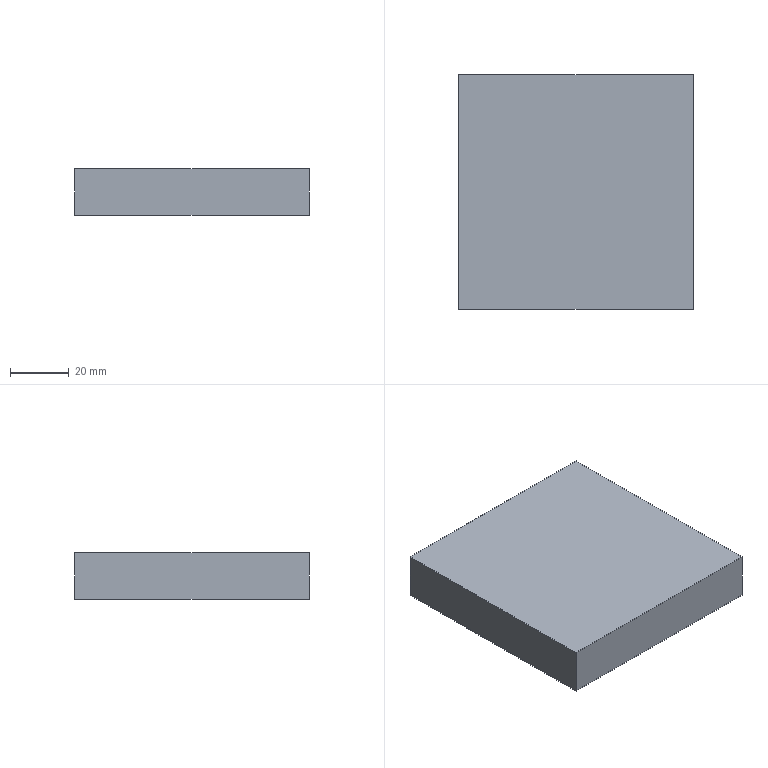Part | SolidWorks | features Chamfer 1, Extrusion 1 | 1 solid | 6 faces | box 80 x 80 x 16 mm | volume 102400 mm3 | plane 6
STEP:
#1=CARTESIAN_POINT('',(40.,-40.,0.));
#2=VERTEX_POINT('',#1);
#3=CARTESIAN_POINT('',(40.,40.,0.));
#4=VERTEX_POINT('',#3);
#5=CARTESIAN_POINT('',(40.,-40.,0.));
#6=DIRECTION('',(0.,1.,0.));
#7=VECTOR('',#6,1000.);
#8=LINE('',#5,#7);
#9=EDGE_CURVE('',#2,#4,#8,.T.);
#10=ORIENTED_EDGE('',*,*,#9,.T.);
#11=CARTESIAN_POINT('',(40.,40.,16.));
#12=VERTEX_POINT('',#11);
#13=CARTESIAN_POINT('',(40.,40.,16.));
#14=DIRECTION('',(0.,0.,-1.));
#15=VECTOR('',#14,1000.);
#16=LINE('',#13,#15);
#17=EDGE_CURVE('',#12,#4,#16,.T.);
#18=ORIENTED_EDGE('',*,*,#17,.F.);
#19=CARTESIAN_POINT('',(40.,-40.,16.));
#20=VERTEX_POINT('',#19);
#21=CARTESIAN_POINT('',(40.,-40.,16.));
#22=DIRECTION('',(0.,1.,0.));
#23=VECTOR('',#22,1000.);
#24=LINE('',#21,#23);
#25=EDGE_CURVE('',#20,#12,#24,.T.);
#26=ORIENTED_EDGE('',*,*,#25,.F.);
#27=CARTESIAN_POINT('',(40.,-40.,16.));
#28=DIRECTION('',(0.,0.,-1.));
#29=VECTOR('',#28,1000.);
#30=LINE('',#27,#29);
#31=EDGE_CURVE('',#20,#2,#30,.T.);
#32=ORIENTED_EDGE('',*,*,#31,.T.);
#33=EDGE_LOOP('',(#10,#18,#26,#32));
#34=FACE_OUTER_BOUND('',#33,.T.);
#35=CARTESIAN_POINT('',(40.,-40.,16.));
#36=DIRECTION('',(-1.,0.,0.));
#37=DIRECTION('',(0.,0.,1.));
#38=AXIS2_PLACEMENT_3D('',#35,#36,#37);
#39=PLANE('',#38);
#40=ADVANCED_FACE('',(#34),#39,.F.);
#41=CARTESIAN_POINT('',(-40.,40.,0.));
#42=VERTEX_POINT('',#41);
#43=CARTESIAN_POINT('',(-40.,40.,0.));
#44=DIRECTION('',(-1.,0.,0.));
#45=VECTOR('',#44,1000.);
#46=LINE('',#43,#45);
#47=EDGE_CURVE('',#4,#42,#46,.T.);
#48=ORIENTED_EDGE('',*,*,#47,.T.);
#49=CARTESIAN_POINT('',(-40.,40.,16.));
#50=VERTEX_POINT('',#49);
#51=CARTESIAN_POINT('',(-40.,40.,16.));
#52=DIRECTION('',(0.,0.,-1.));
#53=VECTOR('',#52,1000.);
#54=LINE('',#51,#53);
#55=EDGE_CURVE('',#50,#42,#54,.T.);
#56=ORIENTED_EDGE('',*,*,#55,.F.);
#57=CARTESIAN_POINT('',(-40.,40.,16.));
#58=DIRECTION('',(-1.,0.,0.));
#59=VECTOR('',#58,1000.);
#60=LINE('',#57,#59);
#61=EDGE_CURVE('',#12,#50,#60,.T.);
#62=ORIENTED_EDGE('',*,*,#61,.F.);
#63=ORIENTED_EDGE('',*,*,#17,.T.);
#64=EDGE_LOOP('',(#48,#56,#62,#63));
#65=FACE_OUTER_BOUND('',#64,.T.);
#66=CARTESIAN_POINT('',(-40.,40.,16.));
#67=DIRECTION('',(0.,-1.,0.));
#68=DIRECTION('',(0.,0.,-1.));
#69=AXIS2_PLACEMENT_3D('',#66,#67,#68);
#70=PLANE('',#69);
#71=ADVANCED_FACE('',(#65),#70,.F.);
#72=CARTESIAN_POINT('',(-40.,-40.,0.));
#73=VERTEX_POINT('',#72);
#74=CARTESIAN_POINT('',(-40.,-40.,0.));
#75=DIRECTION('',(0.,-1.,0.));
#76=VECTOR('',#75,1000.);
#77=LINE('',#74,#76);
#78=EDGE_CURVE('',#42,#73,#77,.T.);
#79=ORIENTED_EDGE('',*,*,#78,.T.);
#80=CARTESIAN_POINT('',(-40.,-40.,16.));
#81=VERTEX_POINT('',#80);
#82=CARTESIAN_POINT('',(-40.,-40.,16.));
#83=DIRECTION('',(0.,0.,-1.));
#84=VECTOR('',#83,1000.);
#85=LINE('',#82,#84);
#86=EDGE_CURVE('',#81,#73,#85,.T.);
#87=ORIENTED_EDGE('',*,*,#86,.F.);
#88=CARTESIAN_POINT('',(-40.,-40.,16.));
#89=DIRECTION('',(0.,-1.,0.));
#90=VECTOR('',#89,1000.);
#91=LINE('',#88,#90);
#92=EDGE_CURVE('',#50,#81,#91,.T.);
#93=ORIENTED_EDGE('',*,*,#92,.F.);
#94=ORIENTED_EDGE('',*,*,#55,.T.);
#95=EDGE_LOOP('',(#79,#87,#93,#94));
#96=FACE_OUTER_BOUND('',#95,.T.);
#97=CARTESIAN_POINT('',(-40.,-40.,16.));
#98=DIRECTION('',(1.,0.,0.));
#99=DIRECTION('',(0.,0.,-1.));
#100=AXIS2_PLACEMENT_3D('',#97,#98,#99);
#101=PLANE('',#100);
#102=ADVANCED_FACE('',(#96),#101,.F.);
#103=CARTESIAN_POINT('',(-40.,-40.,0.));
#104=DIRECTION('',(1.,0.,0.));
#105=VECTOR('',#104,1000.);
#106=LINE('',#103,#105);
#107=EDGE_CURVE('',#73,#2,#106,.T.);
#108=ORIENTED_EDGE('',*,*,#107,.T.);
#109=ORIENTED_EDGE('',*,*,#31,.F.);
#110=CARTESIAN_POINT('',(-40.,-40.,16.));
#111=DIRECTION('',(1.,0.,0.));
#112=VECTOR('',#111,1000.);
#113=LINE('',#110,#112);
#114=EDGE_CURVE('',#81,#20,#113,.T.);
#115=ORIENTED_EDGE('',*,*,#114,.F.);
#116=ORIENTED_EDGE('',*,*,#86,.T.);
#117=EDGE_LOOP('',(#108,#109,#115,#116));
#118=FACE_OUTER_BOUND('',#117,.T.);
#119=CARTESIAN_POINT('',(-40.,-40.,16.));
#120=DIRECTION('',(0.,1.,0.));
#121=DIRECTION('',(0.,0.,1.));
#122=AXIS2_PLACEMENT_3D('',#119,#120,#121);
#123=PLANE('',#122);
#124=ADVANCED_FACE('',(#118),#123,.F.);
#125=ORIENTED_EDGE('',*,*,#25,.T.);
#126=ORIENTED_EDGE('',*,*,#61,.T.);
#127=ORIENTED_EDGE('',*,*,#92,.T.);
#128=ORIENTED_EDGE('',*,*,#114,.T.);
#129=EDGE_LOOP('',(#125,#126,#127,#128));
#130=FACE_OUTER_BOUND('',#129,.T.);
#131=CARTESIAN_POINT('',(0.,0.,16.));
#132=DIRECTION('',(0.,0.,-1.));
#133=DIRECTION('',(-1.,0.,0.));
#134=AXIS2_PLACEMENT_3D('',#131,#132,#133);
#135=PLANE('',#134);
#136=ADVANCED_FACE('',(#130),#135,.F.);
#137=ORIENTED_EDGE('',*,*,#9,.F.);
#138=ORIENTED_EDGE('',*,*,#107,.F.);
#139=ORIENTED_EDGE('',*,*,#78,.F.);
#140=ORIENTED_EDGE('',*,*,#47,.F.);
#141=EDGE_LOOP('',(#137,#138,#139,#140));
#142=FACE_OUTER_BOUND('',#141,.T.);
#143=CARTESIAN_POINT('',(0.,0.,0.));
#144=DIRECTION('',(0.,0.,-1.));
#145=DIRECTION('',(-1.,0.,0.));
#146=AXIS2_PLACEMENT_3D('',#143,#144,#145);
#147=PLANE('',#146);
#148=ADVANCED_FACE('',(#142),#147,.T.);
#149=CLOSED_SHELL('',(#40,#71,#102,#124,#136,#148));
#150=MANIFOLD_SOLID_BREP('',#149);
#151=CARTESIAN_POINT('',(0.,0.,0.));
#152=DIRECTION('',(0.,0.,1.));
#153=DIRECTION('',(1.,0.,0.));
#154=AXIS2_PLACEMENT_3D('',#151,#152,#153);
#155=(LENGTH_UNIT()NAMED_UNIT(*)SI_UNIT(.MILLI.,.METRE.));
#156=UNCERTAINTY_MEASURE_WITH_UNIT(LENGTH_MEASURE(0.00001),#155,'','');
#157=(NAMED_UNIT(*)PLANE_ANGLE_UNIT()SI_UNIT($,.RADIAN.));
#158=(NAMED_UNIT(*)SI_UNIT($,.STERADIAN.)SOLID_ANGLE_UNIT());
#159=(GEOMETRIC_REPRESENTATION_CONTEXT(3)GLOBAL_UNCERTAINTY_ASSIGNED_CONTEXT((#156))GLOBAL_UNIT_ASSIGNED_CONTEXT((#155,#157,#158))REPRESENTATION_CONTEXT('',''));
#160=ADVANCED_BREP_SHAPE_REPRESENTATION('',(#150,#154),#159);